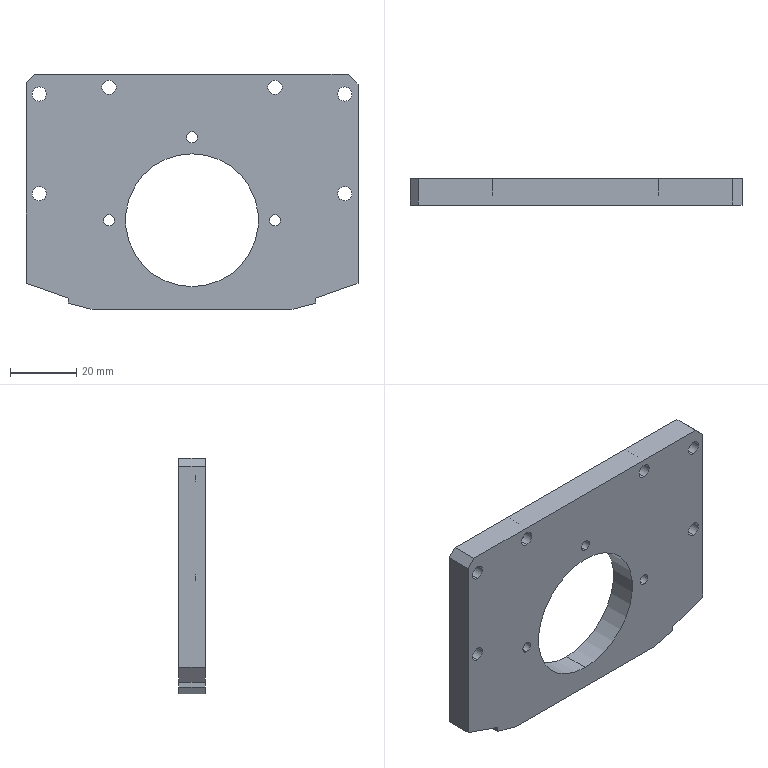Part | STEP file | lead screw Z-axis upper cover plate-direct | 1 solid | 60 faces | box 100 x 8 x 71 mm | volume 43189 mm3 | cylinder 36 | plane 20 | cone 4 | commonest cylinder face diameters 4.3 x12 7.5 x12 3.3 x10 40 x2